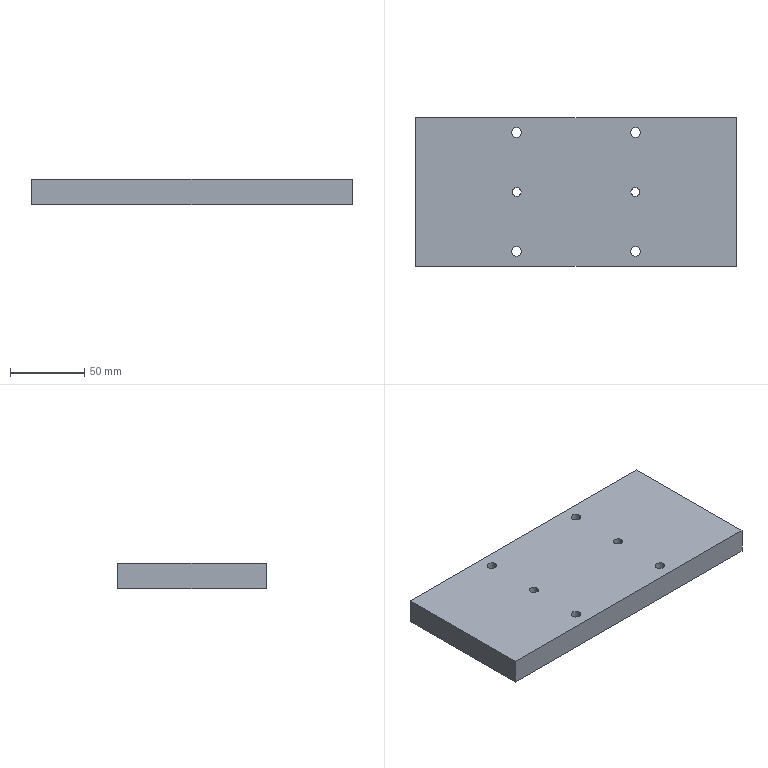Part | SolidWorks | features HoleWzd 2, Extrusion 1 | 1 solid | 30 faces | box 216 x 100 x 17 mm | volume 362258 mm3 | cylinder 20 | plane 10 | commonest cylinder face diameters 6.6 x8 11 x8 6 x4
STEP:
#1=CARTESIAN_POINT('',(-34.5,40.,6.8));
#2=VERTEX_POINT('',#1);
#3=CARTESIAN_POINT('',(-45.5,40.,6.8));
#4=VERTEX_POINT('',#3);
#5=CARTESIAN_POINT('',(-40.,40.,6.8));
#6=DIRECTION('',(0.,0.,-1.));
#7=DIRECTION('',(-1.,0.,0.));
#8=AXIS2_PLACEMENT_3D('',#5,#6,#7);
#9=CIRCLE('',#8,5.5);
#10=EDGE_CURVE('',#2,#4,#9,.T.);
#11=ORIENTED_EDGE('',*,*,#10,.F.);
#12=CARTESIAN_POINT('',(-34.5,40.,0.));
#13=VERTEX_POINT('',#12);
#14=CARTESIAN_POINT('',(-34.5,40.,0.));
#15=DIRECTION('',(0.,0.,-1.));
#16=VECTOR('',#15,1000.);
#17=LINE('',#14,#16);
#18=EDGE_CURVE('',#2,#13,#17,.T.);
#19=ORIENTED_EDGE('',*,*,#18,.T.);
#20=CARTESIAN_POINT('',(-45.5,40.,0.));
#21=VERTEX_POINT('',#20);
#22=CARTESIAN_POINT('',(-40.,40.,0.));
#23=DIRECTION('',(0.,0.,-1.));
#24=DIRECTION('',(-1.,0.,0.));
#25=AXIS2_PLACEMENT_3D('',#22,#23,#24);
#26=CIRCLE('',#25,5.5);
#27=EDGE_CURVE('',#13,#21,#26,.T.);
#28=ORIENTED_EDGE('',*,*,#27,.T.);
#29=CARTESIAN_POINT('',(-45.5,40.,0.));
#30=DIRECTION('',(0.,0.,-1.));
#31=VECTOR('',#30,1000.);
#32=LINE('',#29,#31);
#33=EDGE_CURVE('',#4,#21,#32,.T.);
#34=ORIENTED_EDGE('',*,*,#33,.F.);
#35=EDGE_LOOP('',(#11,#19,#28,#34));
#36=FACE_OUTER_BOUND('',#35,.T.);
#37=CARTESIAN_POINT('',(-40.,40.,0.));
#38=DIRECTION('',(0.,0.,-1.));
#39=DIRECTION('',(-1.,0.,0.));
#40=AXIS2_PLACEMENT_3D('',#37,#38,#39);
#41=CYLINDRICAL_SURFACE('',#40,5.5);
#42=ADVANCED_FACE('',(#36),#41,.F.);
#43=CARTESIAN_POINT('',(-36.7,40.,17.));
#44=VERTEX_POINT('',#43);
#45=CARTESIAN_POINT('',(-43.3,40.,17.));
#46=VERTEX_POINT('',#45);
#47=CARTESIAN_POINT('',(-40.,40.,17.));
#48=DIRECTION('',(0.,0.,-1.));
#49=DIRECTION('',(-1.,0.,0.));
#50=AXIS2_PLACEMENT_3D('',#47,#48,#49);
#51=CIRCLE('',#50,3.3);
#52=EDGE_CURVE('',#44,#46,#51,.T.);
#53=ORIENTED_EDGE('',*,*,#52,.F.);
#54=CARTESIAN_POINT('',(-36.7,40.,6.8));
#55=VERTEX_POINT('',#54);
#56=CARTESIAN_POINT('',(-36.7,40.,0.));
#57=DIRECTION('',(0.,0.,-1.));
#58=VECTOR('',#57,1000.);
#59=LINE('',#56,#58);
#60=EDGE_CURVE('',#44,#55,#59,.T.);
#61=ORIENTED_EDGE('',*,*,#60,.T.);
#62=CARTESIAN_POINT('',(-43.3,40.,6.8));
#63=VERTEX_POINT('',#62);
#64=CARTESIAN_POINT('',(-40.,40.,6.8));
#65=DIRECTION('',(0.,0.,-1.));
#66=DIRECTION('',(-1.,0.,0.));
#67=AXIS2_PLACEMENT_3D('',#64,#65,#66);
#68=CIRCLE('',#67,3.3);
#69=EDGE_CURVE('',#55,#63,#68,.T.);
#70=ORIENTED_EDGE('',*,*,#69,.T.);
#71=CARTESIAN_POINT('',(-43.3,40.,0.));
#72=DIRECTION('',(0.,0.,-1.));
#73=VECTOR('',#72,1000.);
#74=LINE('',#71,#73);
#75=EDGE_CURVE('',#46,#63,#74,.T.);
#76=ORIENTED_EDGE('',*,*,#75,.F.);
#77=EDGE_LOOP('',(#53,#61,#70,#76));
#78=FACE_OUTER_BOUND('',#77,.T.);
#79=CARTESIAN_POINT('',(-40.,40.,0.));
#80=DIRECTION('',(0.,0.,-1.));
#81=DIRECTION('',(-1.,0.,0.));
#82=AXIS2_PLACEMENT_3D('',#79,#80,#81);
#83=CYLINDRICAL_SURFACE('',#82,3.3);
#84=ADVANCED_FACE('',(#78),#83,.F.);
#85=CARTESIAN_POINT('',(-34.5,-40.,6.8));
#86=VERTEX_POINT('',#85);
#87=CARTESIAN_POINT('',(-45.5,-40.,6.8));
#88=VERTEX_POINT('',#87);
#89=CARTESIAN_POINT('',(-40.,-40.,6.8));
#90=DIRECTION('',(0.,0.,-1.));
#91=DIRECTION('',(-1.,0.,0.));
#92=AXIS2_PLACEMENT_3D('',#89,#90,#91);
#93=CIRCLE('',#92,5.5);
#94=EDGE_CURVE('',#86,#88,#93,.T.);
#95=ORIENTED_EDGE('',*,*,#94,.F.);
#96=CARTESIAN_POINT('',(-34.5,-40.,0.));
#97=VERTEX_POINT('',#96);
#98=CARTESIAN_POINT('',(-34.5,-40.,0.));
#99=DIRECTION('',(0.,0.,-1.));
#100=VECTOR('',#99,1000.);
#101=LINE('',#98,#100);
#102=EDGE_CURVE('',#86,#97,#101,.T.);
#103=ORIENTED_EDGE('',*,*,#102,.T.);
#104=CARTESIAN_POINT('',(-45.5,-40.,0.));
#105=VERTEX_POINT('',#104);
#106=CARTESIAN_POINT('',(-40.,-40.,0.));
#107=DIRECTION('',(0.,0.,-1.));
#108=DIRECTION('',(-1.,0.,0.));
#109=AXIS2_PLACEMENT_3D('',#106,#107,#108);
#110=CIRCLE('',#109,5.5);
#111=EDGE_CURVE('',#97,#105,#110,.T.);
#112=ORIENTED_EDGE('',*,*,#111,.T.);
#113=CARTESIAN_POINT('',(-45.5,-40.,0.));
#114=DIRECTION('',(0.,0.,-1.));
#115=VECTOR('',#114,1000.);
#116=LINE('',#113,#115);
#117=EDGE_CURVE('',#88,#105,#116,.T.);
#118=ORIENTED_EDGE('',*,*,#117,.F.);
#119=EDGE_LOOP('',(#95,#103,#112,#118));
#120=FACE_OUTER_BOUND('',#119,.T.);
#121=CARTESIAN_POINT('',(-40.,-40.,0.));
#122=DIRECTION('',(0.,0.,-1.));
#123=DIRECTION('',(-1.,0.,0.));
#124=AXIS2_PLACEMENT_3D('',#121,#122,#123);
#125=CYLINDRICAL_SURFACE('',#124,5.5);
#126=ADVANCED_FACE('',(#120),#125,.F.);
#127=CARTESIAN_POINT('',(-36.7,-40.,17.));
#128=VERTEX_POINT('',#127);
#129=CARTESIAN_POINT('',(-43.3,-40.,17.));
#130=VERTEX_POINT('',#129);
#131=CARTESIAN_POINT('',(-40.,-40.,17.));
#132=DIRECTION('',(0.,0.,-1.));
#133=DIRECTION('',(-1.,0.,0.));
#134=AXIS2_PLACEMENT_3D('',#131,#132,#133);
#135=CIRCLE('',#134,3.3);
#136=EDGE_CURVE('',#128,#130,#135,.T.);
#137=ORIENTED_EDGE('',*,*,#136,.F.);
#138=CARTESIAN_POINT('',(-36.7,-40.,6.8));
#139=VERTEX_POINT('',#138);
#140=CARTESIAN_POINT('',(-36.7,-40.,0.));
#141=DIRECTION('',(0.,0.,-1.));
#142=VECTOR('',#141,1000.);
#143=LINE('',#140,#142);
#144=EDGE_CURVE('',#128,#139,#143,.T.);
#145=ORIENTED_EDGE('',*,*,#144,.T.);
#146=CARTESIAN_POINT('',(-43.3,-40.,6.8));
#147=VERTEX_POINT('',#146);
#148=CARTESIAN_POINT('',(-40.,-40.,6.8));
#149=DIRECTION('',(0.,0.,-1.));
#150=DIRECTION('',(-1.,0.,0.));
#151=AXIS2_PLACEMENT_3D('',#148,#149,#150);
#152=CIRCLE('',#151,3.3);
#153=EDGE_CURVE('',#139,#147,#152,.T.);
#154=ORIENTED_EDGE('',*,*,#153,.T.);
#155=CARTESIAN_POINT('',(-43.3,-40.,0.));
#156=DIRECTION('',(0.,0.,-1.));
#157=VECTOR('',#156,1000.);
#158=LINE('',#155,#157);
#159=EDGE_CURVE('',#130,#147,#158,.T.);
#160=ORIENTED_EDGE('',*,*,#159,.F.);
#161=EDGE_LOOP('',(#137,#145,#154,#160));
#162=FACE_OUTER_BOUND('',#161,.T.);
#163=CARTESIAN_POINT('',(-40.,-40.,0.));
#164=DIRECTION('',(0.,0.,-1.));
#165=DIRECTION('',(-1.,0.,0.));
#166=AXIS2_PLACEMENT_3D('',#163,#164,#165);
#167=CYLINDRICAL_SURFACE('',#166,3.3);
#168=ADVANCED_FACE('',(#162),#167,.F.);
#169=CARTESIAN_POINT('',(45.5,-40.,6.8));
#170=VERTEX_POINT('',#169);
#171=CARTESIAN_POINT('',(34.5,-40.,6.8));
#172=VERTEX_POINT('',#171);
#173=CARTESIAN_POINT('',(40.,-40.,6.8));
#174=DIRECTION('',(0.,0.,-1.));
#175=DIRECTION('',(-1.,0.,0.));
#176=AXIS2_PLACEMENT_3D('',#173,#174,#175);
#177=CIRCLE('',#176,5.5);
#178=EDGE_CURVE('',#170,#172,#177,.T.);
#179=ORIENTED_EDGE('',*,*,#178,.F.);
#180=CARTESIAN_POINT('',(45.5,-40.,0.));
#181=VERTEX_POINT('',#180);
#182=CARTESIAN_POINT('',(45.5,-40.,0.));
#183=DIRECTION('',(0.,0.,-1.));
#184=VECTOR('',#183,1000.);
#185=LINE('',#182,#184);
#186=EDGE_CURVE('',#170,#181,#185,.T.);
#187=ORIENTED_EDGE('',*,*,#186,.T.);
#188=CARTESIAN_POINT('',(34.5,-40.,0.));
#189=VERTEX_POINT('',#188);
#190=CARTESIAN_POINT('',(40.,-40.,0.));
#191=DIRECTION('',(0.,0.,-1.));
#192=DIRECTION('',(-1.,0.,0.));
#193=AXIS2_PLACEMENT_3D('',#190,#191,#192);
#194=CIRCLE('',#193,5.5);
#195=EDGE_CURVE('',#181,#189,#194,.T.);
#196=ORIENTED_EDGE('',*,*,#195,.T.);
#197=CARTESIAN_POINT('',(34.5,-40.,0.));
#198=DIRECTION('',(0.,0.,-1.));
#199=VECTOR('',#198,1000.);
#200=LINE('',#197,#199);
#201=EDGE_CURVE('',#172,#189,#200,.T.);
#202=ORIENTED_EDGE('',*,*,#201,.F.);
#203=EDGE_LOOP('',(#179,#187,#196,#202));
#204=FACE_OUTER_BOUND('',#203,.T.);
#205=CARTESIAN_POINT('',(40.,-40.,0.));
#206=DIRECTION('',(0.,0.,-1.));
#207=DIRECTION('',(-1.,0.,0.));
#208=AXIS2_PLACEMENT_3D('',#205,#206,#207);
#209=CYLINDRICAL_SURFACE('',#208,5.5);
#210=ADVANCED_FACE('',(#204),#209,.F.);
#211=CARTESIAN_POINT('',(43.3,-40.,17.));
#212=VERTEX_POINT('',#211);
#213=CARTESIAN_POINT('',(36.7,-40.,17.));
#214=VERTEX_POINT('',#213);
#215=CARTESIAN_POINT('',(40.,-40.,17.));
#216=DIRECTION('',(0.,0.,-1.));
#217=DIRECTION('',(-1.,0.,0.));
#218=AXIS2_PLACEMENT_3D('',#215,#216,#217);
#219=CIRCLE('',#218,3.3);
#220=EDGE_CURVE('',#212,#214,#219,.T.);
#221=ORIENTED_EDGE('',*,*,#220,.F.);
#222=CARTESIAN_POINT('',(43.3,-40.,6.8));
#223=VERTEX_POINT('',#222);
#224=CARTESIAN_POINT('',(43.3,-40.,0.));
#225=DIRECTION('',(0.,0.,-1.));
#226=VECTOR('',#225,1000.);
#227=LINE('',#224,#226);
#228=EDGE_CURVE('',#212,#223,#227,.T.);
#229=ORIENTED_EDGE('',*,*,#228,.T.);
#230=CARTESIAN_POINT('',(36.7,-40.,6.8));
#231=VERTEX_POINT('',#230);
#232=CARTESIAN_POINT('',(40.,-40.,6.8));
#233=DIRECTION('',(0.,0.,-1.));
#234=DIRECTION('',(-1.,0.,0.));
#235=AXIS2_PLACEMENT_3D('',#232,#233,#234);
#236=CIRCLE('',#235,3.3);
#237=EDGE_CURVE('',#223,#231,#236,.T.);
#238=ORIENTED_EDGE('',*,*,#237,.T.);
#239=CARTESIAN_POINT('',(36.7,-40.,0.));
#240=DIRECTION('',(0.,0.,-1.));
#241=VECTOR('',#240,1000.);
#242=LINE('',#239,#241);
#243=EDGE_CURVE('',#214,#231,#242,.T.);
#244=ORIENTED_EDGE('',*,*,#243,.F.);
#245=EDGE_LOOP('',(#221,#229,#238,#244));
#246=FACE_OUTER_BOUND('',#245,.T.);
#247=CARTESIAN_POINT('',(40.,-40.,0.));
#248=DIRECTION('',(0.,0.,-1.));
#249=DIRECTION('',(-1.,0.,0.));
#250=AXIS2_PLACEMENT_3D('',#247,#248,#249);
#251=CYLINDRICAL_SURFACE('',#250,3.3);
#252=ADVANCED_FACE('',(#246),#251,.F.);
#253=CARTESIAN_POINT('',(45.5,40.,6.8));
#254=VERTEX_POINT('',#253);
#255=CARTESIAN_POINT('',(34.5,40.,6.8));
#256=VERTEX_POINT('',#255);
#257=CARTESIAN_POINT('',(40.,40.,6.8));
#258=DIRECTION('',(0.,0.,-1.));
#259=DIRECTION('',(-1.,0.,0.));
#260=AXIS2_PLACEMENT_3D('',#257,#258,#259);
#261=CIRCLE('',#260,5.5);
#262=EDGE_CURVE('',#254,#256,#261,.T.);
#263=ORIENTED_EDGE('',*,*,#262,.F.);
#264=CARTESIAN_POINT('',(45.5,40.,0.));
#265=VERTEX_POINT('',#264);
#266=CARTESIAN_POINT('',(45.5,40.,0.));
#267=DIRECTION('',(0.,0.,-1.));
#268=VECTOR('',#267,1000.);
#269=LINE('',#266,#268);
#270=EDGE_CURVE('',#254,#265,#269,.T.);
#271=ORIENTED_EDGE('',*,*,#270,.T.);
#272=CARTESIAN_POINT('',(34.5,40.,0.));
#273=VERTEX_POINT('',#272);
#274=CARTESIAN_POINT('',(40.,40.,0.));
#275=DIRECTION('',(0.,0.,-1.));
#276=DIRECTION('',(-1.,0.,0.));
#277=AXIS2_PLACEMENT_3D('',#274,#275,#276);
#278=CIRCLE('',#277,5.5);
#279=EDGE_CURVE('',#265,#273,#278,.T.);
#280=ORIENTED_EDGE('',*,*,#279,.T.);
#281=CARTESIAN_POINT('',(34.5,40.,0.));
#282=DIRECTION('',(0.,0.,-1.));
#283=VECTOR('',#282,1000.);
#284=LINE('',#281,#283);
#285=EDGE_CURVE('',#256,#273,#284,.T.);
#286=ORIENTED_EDGE('',*,*,#285,.F.);
#287=EDGE_LOOP('',(#263,#271,#280,#286));
#288=FACE_OUTER_BOUND('',#287,.T.);
#289=CARTESIAN_POINT('',(40.,40.,0.));
#290=DIRECTION('',(0.,0.,-1.));
#291=DIRECTION('',(-1.,0.,0.));
#292=AXIS2_PLACEMENT_3D('',#289,#290,#291);
#293=CYLINDRICAL_SURFACE('',#292,5.5);
#294=ADVANCED_FACE('',(#288),#293,.F.);
#295=CARTESIAN_POINT('',(43.3,40.,17.));
#296=VERTEX_POINT('',#295);
#297=CARTESIAN_POINT('',(36.7,40.,17.));
#298=VERTEX_POINT('',#297);
#299=CARTESIAN_POINT('',(40.,40.,17.));
#300=DIRECTION('',(0.,0.,-1.));
#301=DIRECTION('',(-1.,0.,0.));
#302=AXIS2_PLACEMENT_3D('',#299,#300,#301);
#303=CIRCLE('',#302,3.3);
#304=EDGE_CURVE('',#296,#298,#303,.T.);
#305=ORIENTED_EDGE('',*,*,#304,.F.);
#306=CARTESIAN_POINT('',(43.3,40.,6.8));
#307=VERTEX_POINT('',#306);
#308=CARTESIAN_POINT('',(43.3,40.,0.));
#309=DIRECTION('',(0.,0.,-1.));
#310=VECTOR('',#309,1000.);
#311=LINE('',#308,#310);
#312=EDGE_CURVE('',#296,#307,#311,.T.);
#313=ORIENTED_EDGE('',*,*,#312,.T.);
#314=CARTESIAN_POINT('',(36.7,40.,6.8));
#315=VERTEX_POINT('',#314);
#316=CARTESIAN_POINT('',(40.,40.,6.8));
#317=DIRECTION('',(0.,0.,-1.));
#318=DIRECTION('',(-1.,0.,0.));
#319=AXIS2_PLACEMENT_3D('',#316,#317,#318);
#320=CIRCLE('',#319,3.3);
#321=EDGE_CURVE('',#307,#315,#320,.T.);
#322=ORIENTED_EDGE('',*,*,#321,.T.);
#323=CARTESIAN_POINT('',(36.7,40.,0.));
#324=DIRECTION('',(0.,0.,-1.));
#325=VECTOR('',#324,1000.);
#326=LINE('',#323,#325);
#327=EDGE_CURVE('',#298,#315,#326,.T.);
#328=ORIENTED_EDGE('',*,*,#327,.F.);
#329=EDGE_LOOP('',(#305,#313,#322,#328));
#330=FACE_OUTER_BOUND('',#329,.T.);
#331=CARTESIAN_POINT('',(40.,40.,0.));
#332=DIRECTION('',(0.,0.,-1.));
#333=DIRECTION('',(-1.,0.,0.));
#334=AXIS2_PLACEMENT_3D('',#331,#332,#333);
#335=CYLINDRICAL_SURFACE('',#334,3.3);
#336=ADVANCED_FACE('',(#330),#335,.F.);
#337=CARTESIAN_POINT('',(43.,0.,17.));
#338=VERTEX_POINT('',#337);
#339=CARTESIAN_POINT('',(37.,0.,17.));
#340=VERTEX_POINT('',#339);
#341=CARTESIAN_POINT('',(40.,0.,17.));
#342=DIRECTION('',(0.,0.,-1.));
#343=DIRECTION('',(-1.,0.,0.));
#344=AXIS2_PLACEMENT_3D('',#341,#342,#343);
#345=CIRCLE('',#344,3.);
#346=EDGE_CURVE('',#338,#340,#345,.T.);
#347=ORIENTED_EDGE('',*,*,#346,.F.);
#348=CARTESIAN_POINT('',(43.,0.,0.));
#349=VERTEX_POINT('',#348);
#350=CARTESIAN_POINT('',(43.,0.,0.));
#351=DIRECTION('',(0.,0.,-1.));
#352=VECTOR('',#351,1000.);
#353=LINE('',#350,#352);
#354=EDGE_CURVE('',#338,#349,#353,.T.);
#355=ORIENTED_EDGE('',*,*,#354,.T.);
#356=CARTESIAN_POINT('',(37.,0.,0.));
#357=VERTEX_POINT('',#356);
#358=CARTESIAN_POINT('',(40.,0.,0.));
#359=DIRECTION('',(0.,0.,-1.));
#360=DIRECTION('',(-1.,0.,0.));
#361=AXIS2_PLACEMENT_3D('',#358,#359,#360);
#362=CIRCLE('',#361,3.);
#363=EDGE_CURVE('',#349,#357,#362,.T.);
#364=ORIENTED_EDGE('',*,*,#363,.T.);
#365=CARTESIAN_POINT('',(37.,0.,0.));
#366=DIRECTION('',(0.,0.,-1.));
#367=VECTOR('',#366,1000.);
#368=LINE('',#365,#367);
#369=EDGE_CURVE('',#340,#357,#368,.T.);
#370=ORIENTED_EDGE('',*,*,#369,.F.);
#371=EDGE_LOOP('',(#347,#355,#364,#370));
#372=FACE_OUTER_BOUND('',#371,.T.);
#373=CARTESIAN_POINT('',(40.,0.,0.));
#374=DIRECTION('',(0.,0.,-1.));
#375=DIRECTION('',(-1.,0.,0.));
#376=AXIS2_PLACEMENT_3D('',#373,#374,#375);
#377=CYLINDRICAL_SURFACE('',#376,3.);
#378=ADVANCED_FACE('',(#372),#377,.F.);
#379=CARTESIAN_POINT('',(-37.,0.,17.));
#380=VERTEX_POINT('',#379);
#381=CARTESIAN_POINT('',(-43.,0.,17.));
#382=VERTEX_POINT('',#381);
#383=CARTESIAN_POINT('',(-40.,0.,17.));
#384=DIRECTION('',(0.,0.,-1.));
#385=DIRECTION('',(-1.,0.,0.));
#386=AXIS2_PLACEMENT_3D('',#383,#384,#385);
#387=CIRCLE('',#386,3.);
#388=EDGE_CURVE('',#380,#382,#387,.T.);
#389=ORIENTED_EDGE('',*,*,#388,.F.);
#390=CARTESIAN_POINT('',(-37.,0.,0.));
#391=VERTEX_POINT('',#390);
#392=CARTESIAN_POINT('',(-37.,0.,0.));
#393=DIRECTION('',(0.,0.,-1.));
#394=VECTOR('',#393,1000.);
#395=LINE('',#392,#394);
#396=EDGE_CURVE('',#380,#391,#395,.T.);
#397=ORIENTED_EDGE('',*,*,#396,.T.);
#398=CARTESIAN_POINT('',(-43.,0.,0.));
#399=VERTEX_POINT('',#398);
#400=CARTESIAN_POINT('',(-40.,0.,0.));
#401=DIRECTION('',(0.,0.,-1.));
#402=DIRECTION('',(-1.,0.,0.));
#403=AXIS2_PLACEMENT_3D('',#400,#401,#402);
#404=CIRCLE('',#403,3.);
#405=EDGE_CURVE('',#391,#399,#404,.T.);
#406=ORIENTED_EDGE('',*,*,#405,.T.);
#407=CARTESIAN_POINT('',(-43.,0.,0.));
#408=DIRECTION('',(0.,0.,-1.));
#409=VECTOR('',#408,1000.);
#410=LINE('',#407,#409);
#411=EDGE_CURVE('',#382,#399,#410,.T.);
#412=ORIENTED_EDGE('',*,*,#411,.F.);
#413=EDGE_LOOP('',(#389,#397,#406,#412));
#414=FACE_OUTER_BOUND('',#413,.T.);
#415=CARTESIAN_POINT('',(-40.,0.,0.));
#416=DIRECTION('',(0.,0.,-1.));
#417=DIRECTION('',(-1.,0.,0.));
#418=AXIS2_PLACEMENT_3D('',#415,#416,#417);
#419=CYLINDRICAL_SURFACE('',#418,3.);
#420=ADVANCED_FACE('',(#414),#419,.F.);
#421=CARTESIAN_POINT('',(-108.,-50.,0.));
#422=VERTEX_POINT('',#421);
#423=CARTESIAN_POINT('',(-108.,50.,0.));
#424=VERTEX_POINT('',#423);
#425=CARTESIAN_POINT('',(-108.,-50.,0.));
#426=DIRECTION('',(0.,1.,0.));
#427=VECTOR('',#426,1000.);
#428=LINE('',#425,#427);
#429=EDGE_CURVE('',#422,#424,#428,.T.);
#430=ORIENTED_EDGE('',*,*,#429,.F.);
#431=CARTESIAN_POINT('',(-108.,-50.,17.));
#432=VERTEX_POINT('',#431);
#433=CARTESIAN_POINT('',(-108.,-50.,17.));
#434=DIRECTION('',(0.,0.,-1.));
#435=VECTOR('',#434,1000.);
#436=LINE('',#433,#435);
#437=EDGE_CURVE('',#432,#422,#436,.T.);
#438=ORIENTED_EDGE('',*,*,#437,.F.);
#439=CARTESIAN_POINT('',(-108.,50.,17.));
#440=VERTEX_POINT('',#439);
#441=CARTESIAN_POINT('',(-108.,-50.,17.));
#442=DIRECTION('',(0.,1.,0.));
#443=VECTOR('',#442,1000.);
#444=LINE('',#441,#443);
#445=EDGE_CURVE('',#432,#440,#444,.T.);
#446=ORIENTED_EDGE('',*,*,#445,.T.);
#447=CARTESIAN_POINT('',(-108.,50.,17.));
#448=DIRECTION('',(0.,0.,-1.));
#449=VECTOR('',#448,1000.);
#450=LINE('',#447,#449);
#451=EDGE_CURVE('',#440,#424,#450,.T.);
#452=ORIENTED_EDGE('',*,*,#451,.T.);
#453=EDGE_LOOP('',(#430,#438,#446,#452));
#454=FACE_OUTER_BOUND('',#453,.T.);
#455=CARTESIAN_POINT('',(-108.,-50.,17.));
#456=DIRECTION('',(-1.,0.,0.));
#457=DIRECTION('',(0.,0.,1.));
#458=AXIS2_PLACEMENT_3D('',#455,#456,#457);
#459=PLANE('',#458);
#460=ADVANCED_FACE('',(#454),#459,.T.);
#461=CARTESIAN_POINT('',(108.,-50.,0.));
#462=VERTEX_POINT('',#461);
#463=CARTESIAN_POINT('',(108.,-50.,0.));
#464=DIRECTION('',(-1.,0.,0.));
#465=VECTOR('',#464,1000.);
#466=LINE('',#463,#465);
#467=EDGE_CURVE('',#462,#422,#466,.T.);
#468=ORIENTED_EDGE('',*,*,#467,.F.);
#469=CARTESIAN_POINT('',(108.,-50.,17.));
#470=VERTEX_POINT('',#469);
#471=CARTESIAN_POINT('',(108.,-50.,17.));
#472=DIRECTION('',(0.,0.,-1.));
#473=VECTOR('',#472,1000.);
#474=LINE('',#471,#473);
#475=EDGE_CURVE('',#470,#462,#474,.T.);
#476=ORIENTED_EDGE('',*,*,#475,.F.);
#477=CARTESIAN_POINT('',(108.,-50.,17.));
#478=DIRECTION('',(-1.,0.,0.));
#479=VECTOR('',#478,1000.);
#480=LINE('',#477,#479);
#481=EDGE_CURVE('',#470,#432,#480,.T.);
#482=ORIENTED_EDGE('',*,*,#481,.T.);
#483=ORIENTED_EDGE('',*,*,#437,.T.);
#484=EDGE_LOOP('',(#468,#476,#482,#483));
#485=FACE_OUTER_BOUND('',#484,.T.);
#486=CARTESIAN_POINT('',(108.,-50.,17.));
#487=DIRECTION('',(0.,-1.,0.));
#488=DIRECTION('',(0.,0.,-1.));
#489=AXIS2_PLACEMENT_3D('',#486,#487,#488);
#490=PLANE('',#489);
#491=ADVANCED_FACE('',(#485),#490,.T.);
#492=CARTESIAN_POINT('',(108.,50.,0.));
#493=VERTEX_POINT('',#492);
#494=CARTESIAN_POINT('',(108.,50.,0.));
#495=DIRECTION('',(0.,-1.,0.));
#496=VECTOR('',#495,1000.);
#497=LINE('',#494,#496);
#498=EDGE_CURVE('',#493,#462,#497,.T.);
#499=ORIENTED_EDGE('',*,*,#498,.F.);
#500=CARTESIAN_POINT('',(108.,50.,17.));
#501=VERTEX_POINT('',#500);
#502=CARTESIAN_POINT('',(108.,50.,17.));
#503=DIRECTION('',(0.,0.,-1.));
#504=VECTOR('',#503,1000.);
#505=LINE('',#502,#504);
#506=EDGE_CURVE('',#501,#493,#505,.T.);
#507=ORIENTED_EDGE('',*,*,#506,.F.);
#508=CARTESIAN_POINT('',(108.,50.,17.));
#509=DIRECTION('',(0.,-1.,0.));
#510=VECTOR('',#509,1000.);
#511=LINE('',#508,#510);
#512=EDGE_CURVE('',#501,#470,#511,.T.);
#513=ORIENTED_EDGE('',*,*,#512,.T.);
#514=ORIENTED_EDGE('',*,*,#475,.T.);
#515=EDGE_LOOP('',(#499,#507,#513,#514));
#516=FACE_OUTER_BOUND('',#515,.T.);
#517=CARTESIAN_POINT('',(108.,50.,17.));
#518=DIRECTION('',(1.,0.,0.));
#519=DIRECTION('',(0.,0.,-1.));
#520=AXIS2_PLACEMENT_3D('',#517,#518,#519);
#521=PLANE('',#520);
#522=ADVANCED_FACE('',(#516),#521,.T.);
#523=CARTESIAN_POINT('',(-108.,50.,0.));
#524=DIRECTION('',(1.,0.,0.));
#525=VECTOR('',#524,1000.);
#526=LINE('',#523,#525);
#527=EDGE_CURVE('',#424,#493,#526,.T.);
#528=ORIENTED_EDGE('',*,*,#527,.F.);
#529=ORIENTED_EDGE('',*,*,#451,.F.);
#530=CARTESIAN_POINT('',(-108.,50.,17.));
#531=DIRECTION('',(1.,0.,0.));
#532=VECTOR('',#531,1000.);
#533=LINE('',#530,#532);
#534=EDGE_CURVE('',#440,#501,#533,.T.);
#535=ORIENTED_EDGE('',*,*,#534,.T.);
#536=ORIENTED_EDGE('',*,*,#506,.T.);
#537=EDGE_LOOP('',(#528,#529,#535,#536));
#538=FACE_OUTER_BOUND('',#537,.T.);
#539=CARTESIAN_POINT('',(-108.,50.,17.));
#540=DIRECTION('',(0.,1.,0.));
#541=DIRECTION('',(0.,0.,1.));
#542=AXIS2_PLACEMENT_3D('',#539,#540,#541);
#543=PLANE('',#542);
#544=ADVANCED_FACE('',(#538),#543,.T.);
#545=CARTESIAN_POINT('',(-40.,40.,17.));
#546=DIRECTION('',(0.,0.,-1.));
#547=DIRECTION('',(-1.,0.,0.));
#548=AXIS2_PLACEMENT_3D('',#545,#546,#547);
#549=CIRCLE('',#548,3.3);
#550=EDGE_CURVE('',#46,#44,#549,.T.);
#551=ORIENTED_EDGE('',*,*,#550,.T.);
#552=ORIENTED_EDGE('',*,*,#52,.T.);
#553=EDGE_LOOP('',(#551,#552));
#554=FACE_BOUND('',#553,.T.);
#555=CARTESIAN_POINT('',(-40.,-40.,17.));
#556=DIRECTION('',(0.,0.,-1.));
#557=DIRECTION('',(-1.,0.,0.));
#558=AXIS2_PLACEMENT_3D('',#555,#556,#557);
#559=CIRCLE('',#558,3.3);
#560=EDGE_CURVE('',#130,#128,#559,.T.);
#561=ORIENTED_EDGE('',*,*,#560,.T.);
#562=ORIENTED_EDGE('',*,*,#136,.T.);
#563=EDGE_LOOP('',(#561,#562));
#564=FACE_BOUND('',#563,.T.);
#565=CARTESIAN_POINT('',(40.,-40.,17.));
#566=DIRECTION('',(0.,0.,-1.));
#567=DIRECTION('',(-1.,0.,0.));
#568=AXIS2_PLACEMENT_3D('',#565,#566,#567);
#569=CIRCLE('',#568,3.3);
#570=EDGE_CURVE('',#214,#212,#569,.T.);
#571=ORIENTED_EDGE('',*,*,#570,.T.);
#572=ORIENTED_EDGE('',*,*,#220,.T.);
#573=EDGE_LOOP('',(#571,#572));
#574=FACE_BOUND('',#573,.T.);
#575=CARTESIAN_POINT('',(40.,40.,17.));
#576=DIRECTION('',(0.,0.,-1.));
#577=DIRECTION('',(-1.,0.,0.));
#578=AXIS2_PLACEMENT_3D('',#575,#576,#577);
#579=CIRCLE('',#578,3.3);
#580=EDGE_CURVE('',#298,#296,#579,.T.);
#581=ORIENTED_EDGE('',*,*,#580,.T.);
#582=ORIENTED_EDGE('',*,*,#304,.T.);
#583=EDGE_LOOP('',(#581,#582));
#584=FACE_BOUND('',#583,.T.);
#585=CARTESIAN_POINT('',(40.,0.,17.));
#586=DIRECTION('',(0.,0.,-1.));
#587=DIRECTION('',(-1.,0.,0.));
#588=AXIS2_PLACEMENT_3D('',#585,#586,#587);
#589=CIRCLE('',#588,3.);
#590=EDGE_CURVE('',#340,#338,#589,.T.);
#591=ORIENTED_EDGE('',*,*,#590,.T.);
#592=ORIENTED_EDGE('',*,*,#346,.T.);
#593=EDGE_LOOP('',(#591,#592));
#594=FACE_BOUND('',#593,.T.);
#595=CARTESIAN_POINT('',(-40.,0.,17.));
#596=DIRECTION('',(0.,0.,-1.));
#597=DIRECTION('',(-1.,0.,0.));
#598=AXIS2_PLACEMENT_3D('',#595,#596,#597);
#599=CIRCLE('',#598,3.);
#600=EDGE_CURVE('',#382,#380,#599,.T.);
#601=ORIENTED_EDGE('',*,*,#600,.T.);
#602=ORIENTED_EDGE('',*,*,#388,.T.);
#603=EDGE_LOOP('',(#601,#602));
#604=FACE_BOUND('',#603,.T.);
#605=ORIENTED_EDGE('',*,*,#445,.F.);
#606=ORIENTED_EDGE('',*,*,#481,.F.);
#607=ORIENTED_EDGE('',*,*,#512,.F.);
#608=ORIENTED_EDGE('',*,*,#534,.F.);
#609=EDGE_LOOP('',(#605,#606,#607,#608));
#610=FACE_OUTER_BOUND('',#609,.T.);
#611=CARTESIAN_POINT('',(0.,0.,17.));
#612=DIRECTION('',(0.,0.,-1.));
#613=DIRECTION('',(-1.,0.,0.));
#614=AXIS2_PLACEMENT_3D('',#611,#612,#613);
#615=PLANE('',#614);
#616=ADVANCED_FACE('',(#554,#564,#574,#584,#594,#604,#610),#615,.F.);
#617=CARTESIAN_POINT('',(-40.,40.,0.));
#618=DIRECTION('',(0.,0.,-1.));
#619=DIRECTION('',(-1.,0.,0.));
#620=AXIS2_PLACEMENT_3D('',#617,#618,#619);
#621=CIRCLE('',#620,5.5);
#622=EDGE_CURVE('',#21,#13,#621,.T.);
#623=ORIENTED_EDGE('',*,*,#622,.F.);
#624=ORIENTED_EDGE('',*,*,#27,.F.);
#625=EDGE_LOOP('',(#623,#624));
#626=FACE_BOUND('',#625,.T.);
#627=CARTESIAN_POINT('',(-40.,-40.,0.));
#628=DIRECTION('',(0.,0.,-1.));
#629=DIRECTION('',(-1.,0.,0.));
#630=AXIS2_PLACEMENT_3D('',#627,#628,#629);
#631=CIRCLE('',#630,5.5);
#632=EDGE_CURVE('',#105,#97,#631,.T.);
#633=ORIENTED_EDGE('',*,*,#632,.F.);
#634=ORIENTED_EDGE('',*,*,#111,.F.);
#635=EDGE_LOOP('',(#633,#634));
#636=FACE_BOUND('',#635,.T.);
#637=CARTESIAN_POINT('',(40.,-40.,0.));
#638=DIRECTION('',(0.,0.,-1.));
#639=DIRECTION('',(-1.,0.,0.));
#640=AXIS2_PLACEMENT_3D('',#637,#638,#639);
#641=CIRCLE('',#640,5.5);
#642=EDGE_CURVE('',#189,#181,#641,.T.);
#643=ORIENTED_EDGE('',*,*,#642,.F.);
#644=ORIENTED_EDGE('',*,*,#195,.F.);
#645=EDGE_LOOP('',(#643,#644));
#646=FACE_BOUND('',#645,.T.);
#647=CARTESIAN_POINT('',(40.,40.,0.));
#648=DIRECTION('',(0.,0.,-1.));
#649=DIRECTION('',(-1.,0.,0.));
#650=AXIS2_PLACEMENT_3D('',#647,#648,#649);
#651=CIRCLE('',#650,5.5);
#652=EDGE_CURVE('',#273,#265,#651,.T.);
#653=ORIENTED_EDGE('',*,*,#652,.F.);
#654=ORIENTED_EDGE('',*,*,#279,.F.);
#655=EDGE_LOOP('',(#653,#654));
#656=FACE_BOUND('',#655,.T.);
#657=CARTESIAN_POINT('',(40.,0.,0.));
#658=DIRECTION('',(0.,0.,-1.));
#659=DIRECTION('',(-1.,0.,0.));
#660=AXIS2_PLACEMENT_3D('',#657,#658,#659);
#661=CIRCLE('',#660,3.);
#662=EDGE_CURVE('',#357,#349,#661,.T.);
#663=ORIENTED_EDGE('',*,*,#662,.F.);
#664=ORIENTED_EDGE('',*,*,#363,.F.);
#665=EDGE_LOOP('',(#663,#664));
#666=FACE_BOUND('',#665,.T.);
#667=CARTESIAN_POINT('',(-40.,0.,0.));
#668=DIRECTION('',(0.,0.,-1.));
#669=DIRECTION('',(-1.,0.,0.));
#670=AXIS2_PLACEMENT_3D('',#667,#668,#669);
#671=CIRCLE('',#670,3.);
#672=EDGE_CURVE('',#399,#391,#671,.T.);
#673=ORIENTED_EDGE('',*,*,#672,.F.);
#674=ORIENTED_EDGE('',*,*,#405,.F.);
#675=EDGE_LOOP('',(#673,#674));
#676=FACE_BOUND('',#675,.T.);
#677=ORIENTED_EDGE('',*,*,#429,.T.);
#678=ORIENTED_EDGE('',*,*,#527,.T.);
#679=ORIENTED_EDGE('',*,*,#498,.T.);
#680=ORIENTED_EDGE('',*,*,#467,.T.);
#681=EDGE_LOOP('',(#677,#678,#679,#680));
#682=FACE_OUTER_BOUND('',#681,.T.);
#683=CARTESIAN_POINT('',(0.,0.,0.));
#684=DIRECTION('',(0.,0.,-1.));
#685=DIRECTION('',(-1.,0.,0.));
#686=AXIS2_PLACEMENT_3D('',#683,#684,#685);
#687=PLANE('',#686);
#688=ADVANCED_FACE('',(#626,#636,#646,#656,#666,#676,#682),#687,.T.);
#689=ORIENTED_EDGE('',*,*,#396,.F.);
#690=ORIENTED_EDGE('',*,*,#600,.F.);
#691=ORIENTED_EDGE('',*,*,#411,.T.);
#692=ORIENTED_EDGE('',*,*,#672,.T.);
#693=EDGE_LOOP('',(#689,#690,#691,#692));
#694=FACE_OUTER_BOUND('',#693,.T.);
#695=CARTESIAN_POINT('',(-40.,0.,0.));
#696=DIRECTION('',(0.,0.,-1.));
#697=DIRECTION('',(-1.,0.,0.));
#698=AXIS2_PLACEMENT_3D('',#695,#696,#697);
#699=CYLINDRICAL_SURFACE('',#698,3.);
#700=ADVANCED_FACE('',(#694),#699,.F.);
#701=ORIENTED_EDGE('',*,*,#354,.F.);
#702=ORIENTED_EDGE('',*,*,#590,.F.);
#703=ORIENTED_EDGE('',*,*,#369,.T.);
#704=ORIENTED_EDGE('',*,*,#662,.T.);
#705=EDGE_LOOP('',(#701,#702,#703,#704));
#706=FACE_OUTER_BOUND('',#705,.T.);
#707=CARTESIAN_POINT('',(40.,0.,0.));
#708=DIRECTION('',(0.,0.,-1.));
#709=DIRECTION('',(-1.,0.,0.));
#710=AXIS2_PLACEMENT_3D('',#707,#708,#709);
#711=CYLINDRICAL_SURFACE('',#710,3.);
#712=ADVANCED_FACE('',(#706),#711,.F.);
#713=ORIENTED_EDGE('',*,*,#312,.F.);
#714=ORIENTED_EDGE('',*,*,#580,.F.);
#715=ORIENTED_EDGE('',*,*,#327,.T.);
#716=CARTESIAN_POINT('',(40.,40.,6.8));
#717=DIRECTION('',(0.,0.,-1.));
#718=DIRECTION('',(-1.,0.,0.));
#719=AXIS2_PLACEMENT_3D('',#716,#717,#718);
#720=CIRCLE('',#719,3.3);
#721=EDGE_CURVE('',#315,#307,#720,.T.);
#722=ORIENTED_EDGE('',*,*,#721,.T.);
#723=EDGE_LOOP('',(#713,#714,#715,#722));
#724=FACE_OUTER_BOUND('',#723,.T.);
#725=CARTESIAN_POINT('',(40.,40.,0.));
#726=DIRECTION('',(0.,0.,-1.));
#727=DIRECTION('',(-1.,0.,0.));
#728=AXIS2_PLACEMENT_3D('',#725,#726,#727);
#729=CYLINDRICAL_SURFACE('',#728,3.3);
#730=ADVANCED_FACE('',(#724),#729,.F.);
#731=ORIENTED_EDGE('',*,*,#721,.F.);
#732=ORIENTED_EDGE('',*,*,#321,.F.);
#733=EDGE_LOOP('',(#731,#732));
#734=FACE_BOUND('',#733,.T.);
#735=CARTESIAN_POINT('',(40.,40.,6.8));
#736=DIRECTION('',(0.,0.,-1.));
#737=DIRECTION('',(-1.,0.,0.));
#738=AXIS2_PLACEMENT_3D('',#735,#736,#737);
#739=CIRCLE('',#738,5.5);
#740=EDGE_CURVE('',#256,#254,#739,.T.);
#741=ORIENTED_EDGE('',*,*,#740,.T.);
#742=ORIENTED_EDGE('',*,*,#262,.T.);
#743=EDGE_LOOP('',(#741,#742));
#744=FACE_OUTER_BOUND('',#743,.T.);
#745=CARTESIAN_POINT('',(43.3,40.,6.8));
#746=DIRECTION('',(0.,0.,1.));
#747=DIRECTION('',(1.,0.,0.));
#748=AXIS2_PLACEMENT_3D('',#745,#746,#747);
#749=PLANE('',#748);
#750=ADVANCED_FACE('',(#734,#744),#749,.F.);
#751=ORIENTED_EDGE('',*,*,#270,.F.);
#752=ORIENTED_EDGE('',*,*,#740,.F.);
#753=ORIENTED_EDGE('',*,*,#285,.T.);
#754=ORIENTED_EDGE('',*,*,#652,.T.);
#755=EDGE_LOOP('',(#751,#752,#753,#754));
#756=FACE_OUTER_BOUND('',#755,.T.);
#757=CARTESIAN_POINT('',(40.,40.,0.));
#758=DIRECTION('',(0.,0.,-1.));
#759=DIRECTION('',(-1.,0.,0.));
#760=AXIS2_PLACEMENT_3D('',#757,#758,#759);
#761=CYLINDRICAL_SURFACE('',#760,5.5);
#762=ADVANCED_FACE('',(#756),#761,.F.);
#763=ORIENTED_EDGE('',*,*,#228,.F.);
#764=ORIENTED_EDGE('',*,*,#570,.F.);
#765=ORIENTED_EDGE('',*,*,#243,.T.);
#766=CARTESIAN_POINT('',(40.,-40.,6.8));
#767=DIRECTION('',(0.,0.,-1.));
#768=DIRECTION('',(-1.,0.,0.));
#769=AXIS2_PLACEMENT_3D('',#766,#767,#768);
#770=CIRCLE('',#769,3.3);
#771=EDGE_CURVE('',#231,#223,#770,.T.);
#772=ORIENTED_EDGE('',*,*,#771,.T.);
#773=EDGE_LOOP('',(#763,#764,#765,#772));
#774=FACE_OUTER_BOUND('',#773,.T.);
#775=CARTESIAN_POINT('',(40.,-40.,0.));
#776=DIRECTION('',(0.,0.,-1.));
#777=DIRECTION('',(-1.,0.,0.));
#778=AXIS2_PLACEMENT_3D('',#775,#776,#777);
#779=CYLINDRICAL_SURFACE('',#778,3.3);
#780=ADVANCED_FACE('',(#774),#779,.F.);
#781=ORIENTED_EDGE('',*,*,#771,.F.);
#782=ORIENTED_EDGE('',*,*,#237,.F.);
#783=EDGE_LOOP('',(#781,#782));
#784=FACE_BOUND('',#783,.T.);
#785=CARTESIAN_POINT('',(40.,-40.,6.8));
#786=DIRECTION('',(0.,0.,-1.));
#787=DIRECTION('',(-1.,0.,0.));
#788=AXIS2_PLACEMENT_3D('',#785,#786,#787);
#789=CIRCLE('',#788,5.5);
#790=EDGE_CURVE('',#172,#170,#789,.T.);
#791=ORIENTED_EDGE('',*,*,#790,.T.);
#792=ORIENTED_EDGE('',*,*,#178,.T.);
#793=EDGE_LOOP('',(#791,#792));
#794=FACE_OUTER_BOUND('',#793,.T.);
#795=CARTESIAN_POINT('',(43.3,-40.,6.8));
#796=DIRECTION('',(0.,0.,1.));
#797=DIRECTION('',(1.,0.,0.));
#798=AXIS2_PLACEMENT_3D('',#795,#796,#797);
#799=PLANE('',#798);
#800=ADVANCED_FACE('',(#784,#794),#799,.F.);
#801=ORIENTED_EDGE('',*,*,#186,.F.);
#802=ORIENTED_EDGE('',*,*,#790,.F.);
#803=ORIENTED_EDGE('',*,*,#201,.T.);
#804=ORIENTED_EDGE('',*,*,#642,.T.);
#805=EDGE_LOOP('',(#801,#802,#803,#804));
#806=FACE_OUTER_BOUND('',#805,.T.);
#807=CARTESIAN_POINT('',(40.,-40.,0.));
#808=DIRECTION('',(0.,0.,-1.));
#809=DIRECTION('',(-1.,0.,0.));
#810=AXIS2_PLACEMENT_3D('',#807,#808,#809);
#811=CYLINDRICAL_SURFACE('',#810,5.5);
#812=ADVANCED_FACE('',(#806),#811,.F.);
#813=ORIENTED_EDGE('',*,*,#144,.F.);
#814=ORIENTED_EDGE('',*,*,#560,.F.);
#815=ORIENTED_EDGE('',*,*,#159,.T.);
#816=CARTESIAN_POINT('',(-40.,-40.,6.8));
#817=DIRECTION('',(0.,0.,-1.));
#818=DIRECTION('',(-1.,0.,0.));
#819=AXIS2_PLACEMENT_3D('',#816,#817,#818);
#820=CIRCLE('',#819,3.3);
#821=EDGE_CURVE('',#147,#139,#820,.T.);
#822=ORIENTED_EDGE('',*,*,#821,.T.);
#823=EDGE_LOOP('',(#813,#814,#815,#822));
#824=FACE_OUTER_BOUND('',#823,.T.);
#825=CARTESIAN_POINT('',(-40.,-40.,0.));
#826=DIRECTION('',(0.,0.,-1.));
#827=DIRECTION('',(-1.,0.,0.));
#828=AXIS2_PLACEMENT_3D('',#825,#826,#827);
#829=CYLINDRICAL_SURFACE('',#828,3.3);
#830=ADVANCED_FACE('',(#824),#829,.F.);
#831=ORIENTED_EDGE('',*,*,#821,.F.);
#832=ORIENTED_EDGE('',*,*,#153,.F.);
#833=EDGE_LOOP('',(#831,#832));
#834=FACE_BOUND('',#833,.T.);
#835=CARTESIAN_POINT('',(-40.,-40.,6.8));
#836=DIRECTION('',(0.,0.,-1.));
#837=DIRECTION('',(-1.,0.,0.));
#838=AXIS2_PLACEMENT_3D('',#835,#836,#837);
#839=CIRCLE('',#838,5.5);
#840=EDGE_CURVE('',#88,#86,#839,.T.);
#841=ORIENTED_EDGE('',*,*,#840,.T.);
#842=ORIENTED_EDGE('',*,*,#94,.T.);
#843=EDGE_LOOP('',(#841,#842));
#844=FACE_OUTER_BOUND('',#843,.T.);
#845=CARTESIAN_POINT('',(-36.7,-40.,6.8));
#846=DIRECTION('',(0.,0.,1.));
#847=DIRECTION('',(1.,0.,0.));
#848=AXIS2_PLACEMENT_3D('',#845,#846,#847);
#849=PLANE('',#848);
#850=ADVANCED_FACE('',(#834,#844),#849,.F.);
#851=ORIENTED_EDGE('',*,*,#102,.F.);
#852=ORIENTED_EDGE('',*,*,#840,.F.);
#853=ORIENTED_EDGE('',*,*,#117,.T.);
#854=ORIENTED_EDGE('',*,*,#632,.T.);
#855=EDGE_LOOP('',(#851,#852,#853,#854));
#856=FACE_OUTER_BOUND('',#855,.T.);
#857=CARTESIAN_POINT('',(-40.,-40.,0.));
#858=DIRECTION('',(0.,0.,-1.));
#859=DIRECTION('',(-1.,0.,0.));
#860=AXIS2_PLACEMENT_3D('',#857,#858,#859);
#861=CYLINDRICAL_SURFACE('',#860,5.5);
#862=ADVANCED_FACE('',(#856),#861,.F.);
#863=ORIENTED_EDGE('',*,*,#60,.F.);
#864=ORIENTED_EDGE('',*,*,#550,.F.);
#865=ORIENTED_EDGE('',*,*,#75,.T.);
#866=CARTESIAN_POINT('',(-40.,40.,6.8));
#867=DIRECTION('',(0.,0.,-1.));
#868=DIRECTION('',(-1.,0.,0.));
#869=AXIS2_PLACEMENT_3D('',#866,#867,#868);
#870=CIRCLE('',#869,3.3);
#871=EDGE_CURVE('',#63,#55,#870,.T.);
#872=ORIENTED_EDGE('',*,*,#871,.T.);
#873=EDGE_LOOP('',(#863,#864,#865,#872));
#874=FACE_OUTER_BOUND('',#873,.T.);
#875=CARTESIAN_POINT('',(-40.,40.,0.));
#876=DIRECTION('',(0.,0.,-1.));
#877=DIRECTION('',(-1.,0.,0.));
#878=AXIS2_PLACEMENT_3D('',#875,#876,#877);
#879=CYLINDRICAL_SURFACE('',#878,3.3);
#880=ADVANCED_FACE('',(#874),#879,.F.);
#881=ORIENTED_EDGE('',*,*,#871,.F.);
#882=ORIENTED_EDGE('',*,*,#69,.F.);
#883=EDGE_LOOP('',(#881,#882));
#884=FACE_BOUND('',#883,.T.);
#885=CARTESIAN_POINT('',(-40.,40.,6.8));
#886=DIRECTION('',(0.,0.,-1.));
#887=DIRECTION('',(-1.,0.,0.));
#888=AXIS2_PLACEMENT_3D('',#885,#886,#887);
#889=CIRCLE('',#888,5.5);
#890=EDGE_CURVE('',#4,#2,#889,.T.);
#891=ORIENTED_EDGE('',*,*,#890,.T.);
#892=ORIENTED_EDGE('',*,*,#10,.T.);
#893=EDGE_LOOP('',(#891,#892));
#894=FACE_OUTER_BOUND('',#893,.T.);
#895=CARTESIAN_POINT('',(-36.7,40.,6.8));
#896=DIRECTION('',(0.,0.,1.));
#897=DIRECTION('',(1.,0.,0.));
#898=AXIS2_PLACEMENT_3D('',#895,#896,#897);
#899=PLANE('',#898);
#900=ADVANCED_FACE('',(#884,#894),#899,.F.);
#901=ORIENTED_EDGE('',*,*,#18,.F.);
#902=ORIENTED_EDGE('',*,*,#890,.F.);
#903=ORIENTED_EDGE('',*,*,#33,.T.);
#904=ORIENTED_EDGE('',*,*,#622,.T.);
#905=EDGE_LOOP('',(#901,#902,#903,#904));
#906=FACE_OUTER_BOUND('',#905,.T.);
#907=CARTESIAN_POINT('',(-40.,40.,0.));
#908=DIRECTION('',(0.,0.,-1.));
#909=DIRECTION('',(-1.,0.,0.));
#910=AXIS2_PLACEMENT_3D('',#907,#908,#909);
#911=CYLINDRICAL_SURFACE('',#910,5.5);
#912=ADVANCED_FACE('',(#906),#911,.F.);
#913=CLOSED_SHELL('',(#42,#84,#126,#168,#210,#252,#294,#336,#378,#420,#460,#491,#522,#544,#616,#688,#700,#712,#730,#750,#762,#780,#800,#812,#830,#850,#862,#880,#900,#912));
#914=MANIFOLD_SOLID_BREP('',#913);
#915=CARTESIAN_POINT('',(0.,0.,0.));
#916=DIRECTION('',(0.,0.,1.));
#917=DIRECTION('',(1.,0.,0.));
#918=AXIS2_PLACEMENT_3D('',#915,#916,#917);
#919=(LENGTH_UNIT()NAMED_UNIT(*)SI_UNIT(.MILLI.,.METRE.));
#920=UNCERTAINTY_MEASURE_WITH_UNIT(LENGTH_MEASURE(0.00001),#919,'','');
#921=(NAMED_UNIT(*)PLANE_ANGLE_UNIT()SI_UNIT($,.RADIAN.));
#922=(NAMED_UNIT(*)SI_UNIT($,.STERADIAN.)SOLID_ANGLE_UNIT());
#923=(GEOMETRIC_REPRESENTATION_CONTEXT(3)GLOBAL_UNCERTAINTY_ASSIGNED_CONTEXT((#920))GLOBAL_UNIT_ASSIGNED_CONTEXT((#919,#921,#922))REPRESENTATION_CONTEXT('',''));
#924=ADVANCED_BREP_SHAPE_REPRESENTATION('',(#914,#918),#923);